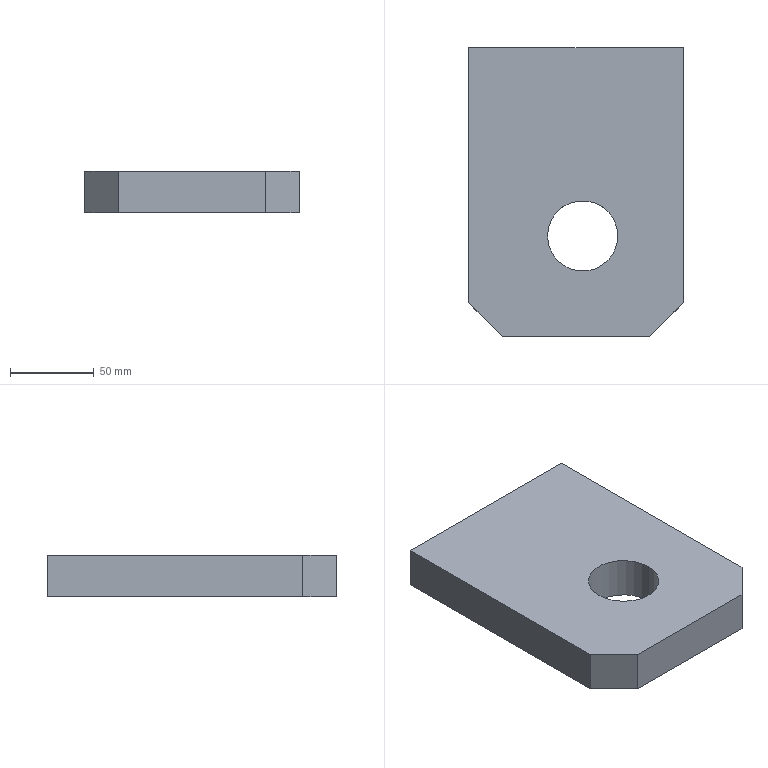Part | STEP file | 08-Plate 2 | 1 solid | 10 faces | box 128 x 172.5 x 25 mm | volume 507364 mm3 | plane 8 | cylinder 2 | commonest cylinder face diameters 42 x2
STEP:
#1=CARTESIAN_POINT('',(0.,0.,0.));
#2=DIRECTION('',(0.,0.,1.));
#3=DIRECTION('',(1.,0.,0.));
#4=AXIS2_PLACEMENT_3D('',#1,#2,#3);
#5=CARTESIAN_POINT('',(89.,-112.5,0.));
#6=VERTEX_POINT('',#5);
#7=CARTESIAN_POINT('',(89.,-112.5,25.));
#8=VERTEX_POINT('',#7);
#9=CARTESIAN_POINT('',(89.,-112.5,-115.));
#10=DIRECTION('',(0.,0.,1.));
#11=VECTOR('',#10,1.);
#12=LINE('',#9,#11);
#13=CARTESIAN_POINT('',(68.,-112.5,-115.));
#14=DIRECTION('',(0.,0.,1.));
#15=DIRECTION('',(1.,0.,0.));
#16=AXIS2_PLACEMENT_3D('',#13,#14,#15);
#17=CYLINDRICAL_SURFACE('',#16,21.);
#18=CARTESIAN_POINT('',(6.283,0.));
#19=DIRECTION('',(0.,1.));
#20=VECTOR('',#19,1.);
#21=LINE('',#18,#20);
#22=(GEOMETRIC_REPRESENTATION_CONTEXT(2)PARAMETRIC_REPRESENTATION_CONTEXT()REPRESENTATION_CONTEXT('',''));
#23=DEFINITIONAL_REPRESENTATION('',(#21),#22);
#24=PCURVE('',#17,#23);
#25=CARTESIAN_POINT('',(68.,-112.5,-115.));
#26=DIRECTION('',(0.,0.,1.));
#27=DIRECTION('',(1.,0.,0.));
#28=AXIS2_PLACEMENT_3D('',#25,#26,#27);
#29=CYLINDRICAL_SURFACE('',#28,21.);
#30=CARTESIAN_POINT('',(0.,0.));
#31=DIRECTION('',(0.,1.));
#32=VECTOR('',#31,1.);
#33=LINE('',#30,#32);
#34=(GEOMETRIC_REPRESENTATION_CONTEXT(2)PARAMETRIC_REPRESENTATION_CONTEXT()REPRESENTATION_CONTEXT('',''));
#35=DEFINITIONAL_REPRESENTATION('',(#33),#34);
#36=PCURVE('',#29,#35);
#37=SURFACE_CURVE('',#12,(#24,#36),.PCURVE_S1.);
#38=EDGE_CURVE('',#6,#8,#37,.T.);
#39=ORIENTED_EDGE('',*,*,#38,.T.);
#40=CARTESIAN_POINT('',(47.,-112.5,25.));
#41=VERTEX_POINT('',#40);
#42=CARTESIAN_POINT('',(68.,-112.5,25.));
#43=DIRECTION('',(0.,0.,1.));
#44=DIRECTION('',(1.,0.,0.));
#45=AXIS2_PLACEMENT_3D('',#42,#43,#44);
#46=CIRCLE('',#45,21.);
#47=CARTESIAN_POINT('',(0.,140.));
#48=DIRECTION('',(1.,0.));
#49=VECTOR('',#48,1.);
#50=LINE('',#47,#49);
#51=(GEOMETRIC_REPRESENTATION_CONTEXT(2)PARAMETRIC_REPRESENTATION_CONTEXT()REPRESENTATION_CONTEXT('',''));
#52=DEFINITIONAL_REPRESENTATION('',(#50),#51);
#53=PCURVE('',#17,#52);
#54=CARTESIAN_POINT('',(0.,0.,25.));
#55=DIRECTION('',(0.,0.,1.));
#56=DIRECTION('',(1.,0.,0.));
#57=AXIS2_PLACEMENT_3D('',#54,#55,#56);
#58=PLANE('',#57);
#59=CARTESIAN_POINT('',(68.,-112.5));
#60=DIRECTION('',(1.,0.));
#61=AXIS2_PLACEMENT_2D('',#59,#60);
#62=CIRCLE('',#61,21.);
#63=(GEOMETRIC_REPRESENTATION_CONTEXT(2)PARAMETRIC_REPRESENTATION_CONTEXT()REPRESENTATION_CONTEXT('',''));
#64=DEFINITIONAL_REPRESENTATION('',(#62),#63);
#65=PCURVE('',#58,#64);
#66=SURFACE_CURVE('',#46,(#53,#65),.PCURVE_S1.);
#67=EDGE_CURVE('',#41,#8,#66,.T.);
#68=ORIENTED_EDGE('',*,*,#67,.F.);
#69=CARTESIAN_POINT('',(47.,-112.5,0.));
#70=VERTEX_POINT('',#69);
#71=CARTESIAN_POINT('',(47.,-112.5,-115.));
#72=DIRECTION('',(0.,0.,1.));
#73=VECTOR('',#72,1.);
#74=LINE('',#71,#73);
#75=CARTESIAN_POINT('',(3.142,0.));
#76=DIRECTION('',(0.,1.));
#77=VECTOR('',#76,1.);
#78=LINE('',#75,#77);
#79=(GEOMETRIC_REPRESENTATION_CONTEXT(2)PARAMETRIC_REPRESENTATION_CONTEXT()REPRESENTATION_CONTEXT('',''));
#80=DEFINITIONAL_REPRESENTATION('',(#78),#79);
#81=PCURVE('',#17,#80);
#82=CARTESIAN_POINT('',(3.142,0.));
#83=DIRECTION('',(0.,1.));
#84=VECTOR('',#83,1.);
#85=LINE('',#82,#84);
#86=(GEOMETRIC_REPRESENTATION_CONTEXT(2)PARAMETRIC_REPRESENTATION_CONTEXT()REPRESENTATION_CONTEXT('',''));
#87=DEFINITIONAL_REPRESENTATION('',(#85),#86);
#88=PCURVE('',#29,#87);
#89=SURFACE_CURVE('',#74,(#81,#88),.PCURVE_S1.);
#90=EDGE_CURVE('',#70,#41,#89,.T.);
#91=ORIENTED_EDGE('',*,*,#90,.F.);
#92=CARTESIAN_POINT('',(68.,-112.5,0.));
#93=DIRECTION('',(0.,0.,1.));
#94=DIRECTION('',(1.,0.,0.));
#95=AXIS2_PLACEMENT_3D('',#92,#93,#94);
#96=CIRCLE('',#95,21.);
#97=CARTESIAN_POINT('',(0.,115.));
#98=DIRECTION('',(1.,0.));
#99=VECTOR('',#98,1.);
#100=LINE('',#97,#99);
#101=(GEOMETRIC_REPRESENTATION_CONTEXT(2)PARAMETRIC_REPRESENTATION_CONTEXT()REPRESENTATION_CONTEXT('',''));
#102=DEFINITIONAL_REPRESENTATION('',(#100),#101);
#103=PCURVE('',#17,#102);
#104=CARTESIAN_POINT('',(0.,0.,0.));
#105=DIRECTION('',(0.,0.,1.));
#106=DIRECTION('',(1.,0.,0.));
#107=AXIS2_PLACEMENT_3D('',#104,#105,#106);
#108=PLANE('',#107);
#109=CARTESIAN_POINT('',(68.,-112.5));
#110=DIRECTION('',(1.,0.));
#111=AXIS2_PLACEMENT_2D('',#109,#110);
#112=CIRCLE('',#111,21.);
#113=(GEOMETRIC_REPRESENTATION_CONTEXT(2)PARAMETRIC_REPRESENTATION_CONTEXT()REPRESENTATION_CONTEXT('',''));
#114=DEFINITIONAL_REPRESENTATION('',(#112),#113);
#115=PCURVE('',#108,#114);
#116=SURFACE_CURVE('',#96,(#103,#115),.PCURVE_S1.);
#117=EDGE_CURVE('',#70,#6,#116,.T.);
#118=ORIENTED_EDGE('',*,*,#117,.T.);
#119=EDGE_LOOP('',(#39,#68,#91,#118));
#120=FACE_BOUND('',#119,.F.);
#121=ADVANCED_FACE('',(#120),#17,.F.);
#122=CARTESIAN_POINT('',(0.,0.,0.));
#123=VERTEX_POINT('',#122);
#124=CARTESIAN_POINT('',(0.,-152.5,0.));
#125=VERTEX_POINT('',#124);
#126=CARTESIAN_POINT('',(0.,0.,0.));
#127=DIRECTION('',(0.,-1.,0.));
#128=VECTOR('',#127,1.);
#129=LINE('',#126,#128);
#130=CARTESIAN_POINT('',(0.,0.,25.));
#131=DIRECTION('',(1.,0.,0.));
#132=DIRECTION('',(0.,1.,0.));
#133=AXIS2_PLACEMENT_3D('',#130,#131,#132);
#134=PLANE('',#133);
#135=CARTESIAN_POINT('',(0.,-25.));
#136=DIRECTION('',(-1.,0.));
#137=VECTOR('',#136,1.);
#138=LINE('',#135,#137);
#139=(GEOMETRIC_REPRESENTATION_CONTEXT(2)PARAMETRIC_REPRESENTATION_CONTEXT()REPRESENTATION_CONTEXT('',''));
#140=DEFINITIONAL_REPRESENTATION('',(#138),#139);
#141=PCURVE('',#134,#140);
#142=CARTESIAN_POINT('',(0.,0.));
#143=DIRECTION('',(0.,-1.));
#144=VECTOR('',#143,1.);
#145=LINE('',#142,#144);
#146=(GEOMETRIC_REPRESENTATION_CONTEXT(2)PARAMETRIC_REPRESENTATION_CONTEXT()REPRESENTATION_CONTEXT('',''));
#147=DEFINITIONAL_REPRESENTATION('',(#145),#146);
#148=PCURVE('',#108,#147);
#149=SURFACE_CURVE('',#129,(#141,#148),.PCURVE_S1.);
#150=EDGE_CURVE('',#123,#125,#149,.T.);
#151=ORIENTED_EDGE('',*,*,#150,.T.);
#152=CARTESIAN_POINT('',(0.,-152.5,25.));
#153=VERTEX_POINT('',#152);
#154=CARTESIAN_POINT('',(0.,-152.5,25.));
#155=DIRECTION('',(0.,0.,1.));
#156=VECTOR('',#155,1.);
#157=LINE('',#154,#156);
#158=CARTESIAN_POINT('',(-152.5,0.));
#159=DIRECTION('',(0.,1.));
#160=VECTOR('',#159,1.);
#161=LINE('',#158,#160);
#162=(GEOMETRIC_REPRESENTATION_CONTEXT(2)PARAMETRIC_REPRESENTATION_CONTEXT()REPRESENTATION_CONTEXT('',''));
#163=DEFINITIONAL_REPRESENTATION('',(#161),#162);
#164=PCURVE('',#134,#163);
#165=CARTESIAN_POINT('',(20.,-172.5,25.));
#166=DIRECTION('',(0.7071,0.7071,0.));
#167=DIRECTION('',(0.,0.,-1.));
#168=AXIS2_PLACEMENT_3D('',#165,#166,#167);
#169=PLANE('',#168);
#170=CARTESIAN_POINT('',(0.,28.284));
#171=DIRECTION('',(-1.,0.));
#172=VECTOR('',#171,1.);
#173=LINE('',#170,#172);
#174=(GEOMETRIC_REPRESENTATION_CONTEXT(2)PARAMETRIC_REPRESENTATION_CONTEXT()REPRESENTATION_CONTEXT('',''));
#175=DEFINITIONAL_REPRESENTATION('',(#173),#174);
#176=PCURVE('',#169,#175);
#177=SURFACE_CURVE('',#157,(#164,#176),.PCURVE_S1.);
#178=EDGE_CURVE('',#125,#153,#177,.T.);
#179=ORIENTED_EDGE('',*,*,#178,.T.);
#180=CARTESIAN_POINT('',(0.,0.,25.));
#181=VERTEX_POINT('',#180);
#182=CARTESIAN_POINT('',(0.,0.,25.));
#183=DIRECTION('',(0.,-1.,0.));
#184=VECTOR('',#183,1.);
#185=LINE('',#182,#184);
#186=CARTESIAN_POINT('',(0.,0.));
#187=DIRECTION('',(-1.,0.));
#188=VECTOR('',#187,1.);
#189=LINE('',#186,#188);
#190=(GEOMETRIC_REPRESENTATION_CONTEXT(2)PARAMETRIC_REPRESENTATION_CONTEXT()REPRESENTATION_CONTEXT('',''));
#191=DEFINITIONAL_REPRESENTATION('',(#189),#190);
#192=PCURVE('',#134,#191);
#193=CARTESIAN_POINT('',(0.,0.));
#194=DIRECTION('',(0.,-1.));
#195=VECTOR('',#194,1.);
#196=LINE('',#193,#195);
#197=(GEOMETRIC_REPRESENTATION_CONTEXT(2)PARAMETRIC_REPRESENTATION_CONTEXT()REPRESENTATION_CONTEXT('',''));
#198=DEFINITIONAL_REPRESENTATION('',(#196),#197);
#199=PCURVE('',#58,#198);
#200=SURFACE_CURVE('',#185,(#192,#199),.PCURVE_S1.);
#201=EDGE_CURVE('',#181,#153,#200,.T.);
#202=ORIENTED_EDGE('',*,*,#201,.F.);
#203=CARTESIAN_POINT('',(0.,0.,25.));
#204=DIRECTION('',(0.,0.,-1.));
#205=VECTOR('',#204,1.);
#206=LINE('',#203,#205);
#207=CARTESIAN_POINT('',(0.,0.));
#208=DIRECTION('',(0.,-1.));
#209=VECTOR('',#208,1.);
#210=LINE('',#207,#209);
#211=(GEOMETRIC_REPRESENTATION_CONTEXT(2)PARAMETRIC_REPRESENTATION_CONTEXT()REPRESENTATION_CONTEXT('',''));
#212=DEFINITIONAL_REPRESENTATION('',(#210),#211);
#213=PCURVE('',#134,#212);
#214=CARTESIAN_POINT('',(0.,0.,25.));
#215=DIRECTION('',(0.,-1.,0.));
#216=DIRECTION('',(0.,0.,-1.));
#217=AXIS2_PLACEMENT_3D('',#214,#215,#216);
#218=PLANE('',#217);
#219=CARTESIAN_POINT('',(0.,0.));
#220=DIRECTION('',(1.,0.));
#221=VECTOR('',#220,1.);
#222=LINE('',#219,#221);
#223=(GEOMETRIC_REPRESENTATION_CONTEXT(2)PARAMETRIC_REPRESENTATION_CONTEXT()REPRESENTATION_CONTEXT('',''));
#224=DEFINITIONAL_REPRESENTATION('',(#222),#223);
#225=PCURVE('',#218,#224);
#226=SURFACE_CURVE('',#206,(#213,#225),.PCURVE_S1.);
#227=EDGE_CURVE('',#181,#123,#226,.T.);
#228=ORIENTED_EDGE('',*,*,#227,.T.);
#229=EDGE_LOOP('',(#151,#179,#202,#228));
#230=FACE_BOUND('',#229,.T.);
#231=ADVANCED_FACE('',(#230),#134,.F.);
#232=CARTESIAN_POINT('',(20.,-172.5,25.));
#233=VERTEX_POINT('',#232);
#234=CARTESIAN_POINT('',(108.,-172.5,25.));
#235=VERTEX_POINT('',#234);
#236=CARTESIAN_POINT('',(0.,-172.5,25.));
#237=DIRECTION('',(1.,0.,0.));
#238=VECTOR('',#237,1.);
#239=LINE('',#236,#238);
#240=CARTESIAN_POINT('',(0.,-172.5,25.));
#241=DIRECTION('',(0.,1.,0.));
#242=DIRECTION('',(0.,0.,1.));
#243=AXIS2_PLACEMENT_3D('',#240,#241,#242);
#244=PLANE('',#243);
#245=CARTESIAN_POINT('',(0.,0.));
#246=DIRECTION('',(0.,1.));
#247=VECTOR('',#246,1.);
#248=LINE('',#245,#247);
#249=(GEOMETRIC_REPRESENTATION_CONTEXT(2)PARAMETRIC_REPRESENTATION_CONTEXT()REPRESENTATION_CONTEXT('',''));
#250=DEFINITIONAL_REPRESENTATION('',(#248),#249);
#251=PCURVE('',#244,#250);
#252=CARTESIAN_POINT('',(0.,-172.5));
#253=DIRECTION('',(1.,0.));
#254=VECTOR('',#253,1.);
#255=LINE('',#252,#254);
#256=(GEOMETRIC_REPRESENTATION_CONTEXT(2)PARAMETRIC_REPRESENTATION_CONTEXT()REPRESENTATION_CONTEXT('',''));
#257=DEFINITIONAL_REPRESENTATION('',(#255),#256);
#258=PCURVE('',#58,#257);
#259=SURFACE_CURVE('',#239,(#251,#258),.PCURVE_S1.);
#260=EDGE_CURVE('',#233,#235,#259,.T.);
#261=ORIENTED_EDGE('',*,*,#260,.F.);
#262=CARTESIAN_POINT('',(20.,-172.5,0.));
#263=VERTEX_POINT('',#262);
#264=CARTESIAN_POINT('',(20.,-172.5,25.));
#265=DIRECTION('',(0.,0.,-1.));
#266=VECTOR('',#265,1.);
#267=LINE('',#264,#266);
#268=CARTESIAN_POINT('',(0.,20.));
#269=DIRECTION('',(-1.,0.));
#270=VECTOR('',#269,1.);
#271=LINE('',#268,#270);
#272=(GEOMETRIC_REPRESENTATION_CONTEXT(2)PARAMETRIC_REPRESENTATION_CONTEXT()REPRESENTATION_CONTEXT('',''));
#273=DEFINITIONAL_REPRESENTATION('',(#271),#272);
#274=PCURVE('',#244,#273);
#275=CARTESIAN_POINT('',(0.,0.));
#276=DIRECTION('',(1.,0.));
#277=VECTOR('',#276,1.);
#278=LINE('',#275,#277);
#279=(GEOMETRIC_REPRESENTATION_CONTEXT(2)PARAMETRIC_REPRESENTATION_CONTEXT()REPRESENTATION_CONTEXT('',''));
#280=DEFINITIONAL_REPRESENTATION('',(#278),#279);
#281=PCURVE('',#169,#280);
#282=SURFACE_CURVE('',#267,(#274,#281),.PCURVE_S1.);
#283=EDGE_CURVE('',#233,#263,#282,.T.);
#284=ORIENTED_EDGE('',*,*,#283,.T.);
#285=CARTESIAN_POINT('',(108.,-172.5,0.));
#286=VERTEX_POINT('',#285);
#287=CARTESIAN_POINT('',(0.,-172.5,0.));
#288=DIRECTION('',(1.,0.,0.));
#289=VECTOR('',#288,1.);
#290=LINE('',#287,#289);
#291=CARTESIAN_POINT('',(-25.,0.));
#292=DIRECTION('',(0.,1.));
#293=VECTOR('',#292,1.);
#294=LINE('',#291,#293);
#295=(GEOMETRIC_REPRESENTATION_CONTEXT(2)PARAMETRIC_REPRESENTATION_CONTEXT()REPRESENTATION_CONTEXT('',''));
#296=DEFINITIONAL_REPRESENTATION('',(#294),#295);
#297=PCURVE('',#244,#296);
#298=CARTESIAN_POINT('',(0.,-172.5));
#299=DIRECTION('',(1.,0.));
#300=VECTOR('',#299,1.);
#301=LINE('',#298,#300);
#302=(GEOMETRIC_REPRESENTATION_CONTEXT(2)PARAMETRIC_REPRESENTATION_CONTEXT()REPRESENTATION_CONTEXT('',''));
#303=DEFINITIONAL_REPRESENTATION('',(#301),#302);
#304=PCURVE('',#108,#303);
#305=SURFACE_CURVE('',#290,(#297,#304),.PCURVE_S1.);
#306=EDGE_CURVE('',#263,#286,#305,.T.);
#307=ORIENTED_EDGE('',*,*,#306,.T.);
#308=CARTESIAN_POINT('',(108.,-172.5,25.));
#309=DIRECTION('',(0.,0.,1.));
#310=VECTOR('',#309,1.);
#311=LINE('',#308,#310);
#312=CARTESIAN_POINT('',(0.,108.));
#313=DIRECTION('',(1.,0.));
#314=VECTOR('',#313,1.);
#315=LINE('',#312,#314);
#316=(GEOMETRIC_REPRESENTATION_CONTEXT(2)PARAMETRIC_REPRESENTATION_CONTEXT()REPRESENTATION_CONTEXT('',''));
#317=DEFINITIONAL_REPRESENTATION('',(#315),#316);
#318=PCURVE('',#244,#317);
#319=CARTESIAN_POINT('',(128.,-152.5,25.));
#320=DIRECTION('',(-0.7071,0.7071,0.));
#321=DIRECTION('',(0.,0.,-1.));
#322=AXIS2_PLACEMENT_3D('',#319,#320,#321);
#323=PLANE('',#322);
#324=CARTESIAN_POINT('',(0.,28.284));
#325=DIRECTION('',(-1.,0.));
#326=VECTOR('',#325,1.);
#327=LINE('',#324,#326);
#328=(GEOMETRIC_REPRESENTATION_CONTEXT(2)PARAMETRIC_REPRESENTATION_CONTEXT()REPRESENTATION_CONTEXT('',''));
#329=DEFINITIONAL_REPRESENTATION('',(#327),#328);
#330=PCURVE('',#323,#329);
#331=SURFACE_CURVE('',#311,(#318,#330),.PCURVE_S1.);
#332=EDGE_CURVE('',#286,#235,#331,.T.);
#333=ORIENTED_EDGE('',*,*,#332,.T.);
#334=EDGE_LOOP('',(#261,#284,#307,#333));
#335=FACE_BOUND('',#334,.T.);
#336=ADVANCED_FACE('',(#335),#244,.F.);
#337=CARTESIAN_POINT('',(128.,-152.5,25.));
#338=VERTEX_POINT('',#337);
#339=CARTESIAN_POINT('',(128.,0.,25.));
#340=VERTEX_POINT('',#339);
#341=CARTESIAN_POINT('',(128.,0.,25.));
#342=DIRECTION('',(0.,1.,0.));
#343=VECTOR('',#342,1.);
#344=LINE('',#341,#343);
#345=CARTESIAN_POINT('',(128.,0.,25.));
#346=DIRECTION('',(-1.,0.,0.));
#347=DIRECTION('',(0.,-1.,0.));
#348=AXIS2_PLACEMENT_3D('',#345,#346,#347);
#349=PLANE('',#348);
#350=CARTESIAN_POINT('',(0.,0.));
#351=DIRECTION('',(-1.,0.));
#352=VECTOR('',#351,1.);
#353=LINE('',#350,#352);
#354=(GEOMETRIC_REPRESENTATION_CONTEXT(2)PARAMETRIC_REPRESENTATION_CONTEXT()REPRESENTATION_CONTEXT('',''));
#355=DEFINITIONAL_REPRESENTATION('',(#353),#354);
#356=PCURVE('',#349,#355);
#357=CARTESIAN_POINT('',(128.,0.));
#358=DIRECTION('',(0.,1.));
#359=VECTOR('',#358,1.);
#360=LINE('',#357,#359);
#361=(GEOMETRIC_REPRESENTATION_CONTEXT(2)PARAMETRIC_REPRESENTATION_CONTEXT()REPRESENTATION_CONTEXT('',''));
#362=DEFINITIONAL_REPRESENTATION('',(#360),#361);
#363=PCURVE('',#58,#362);
#364=SURFACE_CURVE('',#344,(#356,#363),.PCURVE_S1.);
#365=EDGE_CURVE('',#338,#340,#364,.T.);
#366=ORIENTED_EDGE('',*,*,#365,.F.);
#367=CARTESIAN_POINT('',(128.,-152.5,0.));
#368=VERTEX_POINT('',#367);
#369=CARTESIAN_POINT('',(128.,-152.5,25.));
#370=DIRECTION('',(0.,0.,-1.));
#371=VECTOR('',#370,1.);
#372=LINE('',#369,#371);
#373=CARTESIAN_POINT('',(152.5,0.));
#374=DIRECTION('',(0.,-1.));
#375=VECTOR('',#374,1.);
#376=LINE('',#373,#375);
#377=(GEOMETRIC_REPRESENTATION_CONTEXT(2)PARAMETRIC_REPRESENTATION_CONTEXT()REPRESENTATION_CONTEXT('',''));
#378=DEFINITIONAL_REPRESENTATION('',(#376),#377);
#379=PCURVE('',#349,#378);
#380=CARTESIAN_POINT('',(0.,0.));
#381=DIRECTION('',(1.,0.));
#382=VECTOR('',#381,1.);
#383=LINE('',#380,#382);
#384=(GEOMETRIC_REPRESENTATION_CONTEXT(2)PARAMETRIC_REPRESENTATION_CONTEXT()REPRESENTATION_CONTEXT('',''));
#385=DEFINITIONAL_REPRESENTATION('',(#383),#384);
#386=PCURVE('',#323,#385);
#387=SURFACE_CURVE('',#372,(#379,#386),.PCURVE_S1.);
#388=EDGE_CURVE('',#338,#368,#387,.T.);
#389=ORIENTED_EDGE('',*,*,#388,.T.);
#390=CARTESIAN_POINT('',(128.,0.,0.));
#391=VERTEX_POINT('',#390);
#392=CARTESIAN_POINT('',(128.,0.,0.));
#393=DIRECTION('',(0.,1.,0.));
#394=VECTOR('',#393,1.);
#395=LINE('',#392,#394);
#396=CARTESIAN_POINT('',(0.,-25.));
#397=DIRECTION('',(-1.,0.));
#398=VECTOR('',#397,1.);
#399=LINE('',#396,#398);
#400=(GEOMETRIC_REPRESENTATION_CONTEXT(2)PARAMETRIC_REPRESENTATION_CONTEXT()REPRESENTATION_CONTEXT('',''));
#401=DEFINITIONAL_REPRESENTATION('',(#399),#400);
#402=PCURVE('',#349,#401);
#403=CARTESIAN_POINT('',(128.,0.));
#404=DIRECTION('',(0.,1.));
#405=VECTOR('',#404,1.);
#406=LINE('',#403,#405);
#407=(GEOMETRIC_REPRESENTATION_CONTEXT(2)PARAMETRIC_REPRESENTATION_CONTEXT()REPRESENTATION_CONTEXT('',''));
#408=DEFINITIONAL_REPRESENTATION('',(#406),#407);
#409=PCURVE('',#108,#408);
#410=SURFACE_CURVE('',#395,(#402,#409),.PCURVE_S1.);
#411=EDGE_CURVE('',#368,#391,#410,.T.);
#412=ORIENTED_EDGE('',*,*,#411,.T.);
#413=CARTESIAN_POINT('',(128.,0.,25.));
#414=DIRECTION('',(0.,0.,-1.));
#415=VECTOR('',#414,1.);
#416=LINE('',#413,#415);
#417=CARTESIAN_POINT('',(0.,0.));
#418=DIRECTION('',(0.,-1.));
#419=VECTOR('',#418,1.);
#420=LINE('',#417,#419);
#421=(GEOMETRIC_REPRESENTATION_CONTEXT(2)PARAMETRIC_REPRESENTATION_CONTEXT()REPRESENTATION_CONTEXT('',''));
#422=DEFINITIONAL_REPRESENTATION('',(#420),#421);
#423=PCURVE('',#349,#422);
#424=CARTESIAN_POINT('',(0.,128.));
#425=DIRECTION('',(1.,0.));
#426=VECTOR('',#425,1.);
#427=LINE('',#424,#426);
#428=(GEOMETRIC_REPRESENTATION_CONTEXT(2)PARAMETRIC_REPRESENTATION_CONTEXT()REPRESENTATION_CONTEXT('',''));
#429=DEFINITIONAL_REPRESENTATION('',(#427),#428);
#430=PCURVE('',#218,#429);
#431=SURFACE_CURVE('',#416,(#423,#430),.PCURVE_S1.);
#432=EDGE_CURVE('',#340,#391,#431,.T.);
#433=ORIENTED_EDGE('',*,*,#432,.F.);
#434=EDGE_LOOP('',(#366,#389,#412,#433));
#435=FACE_BOUND('',#434,.T.);
#436=ADVANCED_FACE('',(#435),#349,.F.);
#437=CARTESIAN_POINT('',(0.,0.,0.));
#438=DIRECTION('',(-1.,0.,0.));
#439=VECTOR('',#438,1.);
#440=LINE('',#437,#439);
#441=CARTESIAN_POINT('',(25.,0.));
#442=DIRECTION('',(0.,-1.));
#443=VECTOR('',#442,1.);
#444=LINE('',#441,#443);
#445=(GEOMETRIC_REPRESENTATION_CONTEXT(2)PARAMETRIC_REPRESENTATION_CONTEXT()REPRESENTATION_CONTEXT('',''));
#446=DEFINITIONAL_REPRESENTATION('',(#444),#445);
#447=PCURVE('',#218,#446);
#448=CARTESIAN_POINT('',(0.,0.));
#449=DIRECTION('',(-1.,0.));
#450=VECTOR('',#449,1.);
#451=LINE('',#448,#450);
#452=(GEOMETRIC_REPRESENTATION_CONTEXT(2)PARAMETRIC_REPRESENTATION_CONTEXT()REPRESENTATION_CONTEXT('',''));
#453=DEFINITIONAL_REPRESENTATION('',(#451),#452);
#454=PCURVE('',#108,#453);
#455=SURFACE_CURVE('',#440,(#447,#454),.PCURVE_S1.);
#456=EDGE_CURVE('',#391,#123,#455,.T.);
#457=ORIENTED_EDGE('',*,*,#456,.T.);
#458=ORIENTED_EDGE('',*,*,#227,.F.);
#459=CARTESIAN_POINT('',(0.,0.,25.));
#460=DIRECTION('',(-1.,0.,0.));
#461=VECTOR('',#460,1.);
#462=LINE('',#459,#461);
#463=CARTESIAN_POINT('',(0.,0.));
#464=DIRECTION('',(0.,-1.));
#465=VECTOR('',#464,1.);
#466=LINE('',#463,#465);
#467=(GEOMETRIC_REPRESENTATION_CONTEXT(2)PARAMETRIC_REPRESENTATION_CONTEXT()REPRESENTATION_CONTEXT('',''));
#468=DEFINITIONAL_REPRESENTATION('',(#466),#467);
#469=PCURVE('',#218,#468);
#470=CARTESIAN_POINT('',(0.,0.));
#471=DIRECTION('',(-1.,0.));
#472=VECTOR('',#471,1.);
#473=LINE('',#470,#472);
#474=(GEOMETRIC_REPRESENTATION_CONTEXT(2)PARAMETRIC_REPRESENTATION_CONTEXT()REPRESENTATION_CONTEXT('',''));
#475=DEFINITIONAL_REPRESENTATION('',(#473),#474);
#476=PCURVE('',#58,#475);
#477=SURFACE_CURVE('',#462,(#469,#476),.PCURVE_S1.);
#478=EDGE_CURVE('',#340,#181,#477,.T.);
#479=ORIENTED_EDGE('',*,*,#478,.F.);
#480=ORIENTED_EDGE('',*,*,#432,.T.);
#481=EDGE_LOOP('',(#457,#458,#479,#480));
#482=FACE_BOUND('',#481,.T.);
#483=ADVANCED_FACE('',(#482),#218,.F.);
#484=CARTESIAN_POINT('',(68.,-112.5,25.));
#485=DIRECTION('',(0.,0.,1.));
#486=DIRECTION('',(1.,0.,0.));
#487=AXIS2_PLACEMENT_3D('',#484,#485,#486);
#488=CIRCLE('',#487,21.);
#489=CARTESIAN_POINT('',(68.,-112.5));
#490=DIRECTION('',(1.,0.));
#491=AXIS2_PLACEMENT_2D('',#489,#490);
#492=CIRCLE('',#491,21.);
#493=(GEOMETRIC_REPRESENTATION_CONTEXT(2)PARAMETRIC_REPRESENTATION_CONTEXT()REPRESENTATION_CONTEXT('',''));
#494=DEFINITIONAL_REPRESENTATION('',(#492),#493);
#495=PCURVE('',#58,#494);
#496=CARTESIAN_POINT('',(0.,140.));
#497=DIRECTION('',(1.,0.));
#498=VECTOR('',#497,1.);
#499=LINE('',#496,#498);
#500=(GEOMETRIC_REPRESENTATION_CONTEXT(2)PARAMETRIC_REPRESENTATION_CONTEXT()REPRESENTATION_CONTEXT('',''));
#501=DEFINITIONAL_REPRESENTATION('',(#499),#500);
#502=PCURVE('',#29,#501);
#503=SURFACE_CURVE('',#488,(#495,#502),.PCURVE_S1.);
#504=EDGE_CURVE('',#8,#41,#503,.T.);
#505=ORIENTED_EDGE('',*,*,#504,.F.);
#506=ORIENTED_EDGE('',*,*,#67,.F.);
#507=EDGE_LOOP('',(#505,#506));
#508=FACE_BOUND('',#507,.T.);
#509=ORIENTED_EDGE('',*,*,#201,.T.);
#510=CARTESIAN_POINT('',(-76.25,-76.25,25.));
#511=DIRECTION('',(0.7071,-0.7071,0.));
#512=VECTOR('',#511,1.);
#513=LINE('',#510,#512);
#514=CARTESIAN_POINT('',(-76.25,-76.25));
#515=DIRECTION('',(0.7071,-0.7071));
#516=VECTOR('',#515,1.);
#517=LINE('',#514,#516);
#518=(GEOMETRIC_REPRESENTATION_CONTEXT(2)PARAMETRIC_REPRESENTATION_CONTEXT()REPRESENTATION_CONTEXT('',''));
#519=DEFINITIONAL_REPRESENTATION('',(#517),#518);
#520=PCURVE('',#58,#519);
#521=CARTESIAN_POINT('',(0.,136.118));
#522=DIRECTION('',(0.,-1.));
#523=VECTOR('',#522,1.);
#524=LINE('',#521,#523);
#525=(GEOMETRIC_REPRESENTATION_CONTEXT(2)PARAMETRIC_REPRESENTATION_CONTEXT()REPRESENTATION_CONTEXT('',''));
#526=DEFINITIONAL_REPRESENTATION('',(#524),#525);
#527=PCURVE('',#169,#526);
#528=SURFACE_CURVE('',#513,(#520,#527),.PCURVE_S1.);
#529=EDGE_CURVE('',#153,#233,#528,.T.);
#530=ORIENTED_EDGE('',*,*,#529,.T.);
#531=ORIENTED_EDGE('',*,*,#260,.T.);
#532=CARTESIAN_POINT('',(140.25,-140.25,25.));
#533=DIRECTION('',(0.7071,0.7071,0.));
#534=VECTOR('',#533,1.);
#535=LINE('',#532,#534);
#536=CARTESIAN_POINT('',(140.25,-140.25));
#537=DIRECTION('',(0.7071,0.7071));
#538=VECTOR('',#537,1.);
#539=LINE('',#536,#538);
#540=(GEOMETRIC_REPRESENTATION_CONTEXT(2)PARAMETRIC_REPRESENTATION_CONTEXT()REPRESENTATION_CONTEXT('',''));
#541=DEFINITIONAL_REPRESENTATION('',(#539),#540);
#542=PCURVE('',#58,#541);
#543=CARTESIAN_POINT('',(0.,-17.324));
#544=DIRECTION('',(0.,-1.));
#545=VECTOR('',#544,1.);
#546=LINE('',#543,#545);
#547=(GEOMETRIC_REPRESENTATION_CONTEXT(2)PARAMETRIC_REPRESENTATION_CONTEXT()REPRESENTATION_CONTEXT('',''));
#548=DEFINITIONAL_REPRESENTATION('',(#546),#547);
#549=PCURVE('',#323,#548);
#550=SURFACE_CURVE('',#535,(#542,#549),.PCURVE_S1.);
#551=EDGE_CURVE('',#235,#338,#550,.T.);
#552=ORIENTED_EDGE('',*,*,#551,.T.);
#553=ORIENTED_EDGE('',*,*,#365,.T.);
#554=ORIENTED_EDGE('',*,*,#478,.T.);
#555=EDGE_LOOP('',(#509,#530,#531,#552,#553,#554));
#556=FACE_BOUND('',#555,.T.);
#557=ADVANCED_FACE('',(#508,#556),#58,.T.);
#558=CARTESIAN_POINT('',(68.,-112.5,0.));
#559=DIRECTION('',(0.,0.,1.));
#560=DIRECTION('',(1.,0.,0.));
#561=AXIS2_PLACEMENT_3D('',#558,#559,#560);
#562=CIRCLE('',#561,21.);
#563=CARTESIAN_POINT('',(68.,-112.5));
#564=DIRECTION('',(1.,0.));
#565=AXIS2_PLACEMENT_2D('',#563,#564);
#566=CIRCLE('',#565,21.);
#567=(GEOMETRIC_REPRESENTATION_CONTEXT(2)PARAMETRIC_REPRESENTATION_CONTEXT()REPRESENTATION_CONTEXT('',''));
#568=DEFINITIONAL_REPRESENTATION('',(#566),#567);
#569=PCURVE('',#108,#568);
#570=CARTESIAN_POINT('',(0.,115.));
#571=DIRECTION('',(1.,0.));
#572=VECTOR('',#571,1.);
#573=LINE('',#570,#572);
#574=(GEOMETRIC_REPRESENTATION_CONTEXT(2)PARAMETRIC_REPRESENTATION_CONTEXT()REPRESENTATION_CONTEXT('',''));
#575=DEFINITIONAL_REPRESENTATION('',(#573),#574);
#576=PCURVE('',#29,#575);
#577=SURFACE_CURVE('',#562,(#569,#576),.PCURVE_S1.);
#578=EDGE_CURVE('',#6,#70,#577,.T.);
#579=ORIENTED_EDGE('',*,*,#578,.T.);
#580=ORIENTED_EDGE('',*,*,#117,.T.);
#581=EDGE_LOOP('',(#579,#580));
#582=FACE_BOUND('',#581,.T.);
#583=ORIENTED_EDGE('',*,*,#306,.F.);
#584=CARTESIAN_POINT('',(20.,-172.5,0.));
#585=DIRECTION('',(-0.7071,0.7071,0.));
#586=VECTOR('',#585,1.);
#587=LINE('',#584,#586);
#588=CARTESIAN_POINT('',(20.,-172.5));
#589=DIRECTION('',(-0.7071,0.7071));
#590=VECTOR('',#589,1.);
#591=LINE('',#588,#590);
#592=(GEOMETRIC_REPRESENTATION_CONTEXT(2)PARAMETRIC_REPRESENTATION_CONTEXT()REPRESENTATION_CONTEXT('',''));
#593=DEFINITIONAL_REPRESENTATION('',(#591),#592);
#594=PCURVE('',#108,#593);
#595=CARTESIAN_POINT('',(25.,0.));
#596=DIRECTION('',(0.,1.));
#597=VECTOR('',#596,1.);
#598=LINE('',#595,#597);
#599=(GEOMETRIC_REPRESENTATION_CONTEXT(2)PARAMETRIC_REPRESENTATION_CONTEXT()REPRESENTATION_CONTEXT('',''));
#600=DEFINITIONAL_REPRESENTATION('',(#598),#599);
#601=PCURVE('',#169,#600);
#602=SURFACE_CURVE('',#587,(#594,#601),.PCURVE_S1.);
#603=EDGE_CURVE('',#263,#125,#602,.T.);
#604=ORIENTED_EDGE('',*,*,#603,.T.);
#605=ORIENTED_EDGE('',*,*,#150,.F.);
#606=ORIENTED_EDGE('',*,*,#456,.F.);
#607=ORIENTED_EDGE('',*,*,#411,.F.);
#608=CARTESIAN_POINT('',(128.,-152.5,0.));
#609=DIRECTION('',(-0.7071,-0.7071,0.));
#610=VECTOR('',#609,1.);
#611=LINE('',#608,#610);
#612=CARTESIAN_POINT('',(128.,-152.5));
#613=DIRECTION('',(-0.7071,-0.7071));
#614=VECTOR('',#613,1.);
#615=LINE('',#612,#614);
#616=(GEOMETRIC_REPRESENTATION_CONTEXT(2)PARAMETRIC_REPRESENTATION_CONTEXT()REPRESENTATION_CONTEXT('',''));
#617=DEFINITIONAL_REPRESENTATION('',(#615),#616);
#618=PCURVE('',#108,#617);
#619=CARTESIAN_POINT('',(25.,0.));
#620=DIRECTION('',(0.,1.));
#621=VECTOR('',#620,1.);
#622=LINE('',#619,#621);
#623=(GEOMETRIC_REPRESENTATION_CONTEXT(2)PARAMETRIC_REPRESENTATION_CONTEXT()REPRESENTATION_CONTEXT('',''));
#624=DEFINITIONAL_REPRESENTATION('',(#622),#623);
#625=PCURVE('',#323,#624);
#626=SURFACE_CURVE('',#611,(#618,#625),.PCURVE_S1.);
#627=EDGE_CURVE('',#368,#286,#626,.T.);
#628=ORIENTED_EDGE('',*,*,#627,.T.);
#629=EDGE_LOOP('',(#583,#604,#605,#606,#607,#628));
#630=FACE_BOUND('',#629,.T.);
#631=ADVANCED_FACE('',(#582,#630),#108,.F.);
#632=ORIENTED_EDGE('',*,*,#529,.F.);
#633=ORIENTED_EDGE('',*,*,#178,.F.);
#634=ORIENTED_EDGE('',*,*,#603,.F.);
#635=ORIENTED_EDGE('',*,*,#283,.F.);
#636=EDGE_LOOP('',(#632,#633,#634,#635));
#637=FACE_BOUND('',#636,.T.);
#638=ADVANCED_FACE('',(#637),#169,.F.);
#639=ORIENTED_EDGE('',*,*,#551,.F.);
#640=ORIENTED_EDGE('',*,*,#332,.F.);
#641=ORIENTED_EDGE('',*,*,#627,.F.);
#642=ORIENTED_EDGE('',*,*,#388,.F.);
#643=EDGE_LOOP('',(#639,#640,#641,#642));
#644=FACE_BOUND('',#643,.T.);
#645=ADVANCED_FACE('',(#644),#323,.F.);
#646=ORIENTED_EDGE('',*,*,#504,.F.);
#647=ORIENTED_EDGE('',*,*,#38,.F.);
#648=ORIENTED_EDGE('',*,*,#578,.T.);
#649=ORIENTED_EDGE('',*,*,#90,.T.);
#650=EDGE_LOOP('',(#646,#647,#648,#649));
#651=FACE_BOUND('',#650,.F.);
#652=ADVANCED_FACE('',(#651),#29,.F.);
#653=CLOSED_SHELL('',(#121,#231,#336,#436,#483,#557,#631,#638,#645,#652));
#654=MANIFOLD_SOLID_BREP('',#653);
#655=(LENGTH_UNIT()NAMED_UNIT(*)SI_UNIT(.MILLI.,.METRE.));
#656=UNCERTAINTY_MEASURE_WITH_UNIT(LENGTH_MEASURE(0.0000001),#655,'','');
#657=(NAMED_UNIT(*)PLANE_ANGLE_UNIT()SI_UNIT($,.RADIAN.));
#658=(NAMED_UNIT(*)SI_UNIT($,.STERADIAN.)SOLID_ANGLE_UNIT());
#659=(GEOMETRIC_REPRESENTATION_CONTEXT(3)GLOBAL_UNCERTAINTY_ASSIGNED_CONTEXT((#656))GLOBAL_UNIT_ASSIGNED_CONTEXT((#655,#657,#658))REPRESENTATION_CONTEXT('',''));
#660=ADVANCED_BREP_SHAPE_REPRESENTATION('',(#4,#654),#659);